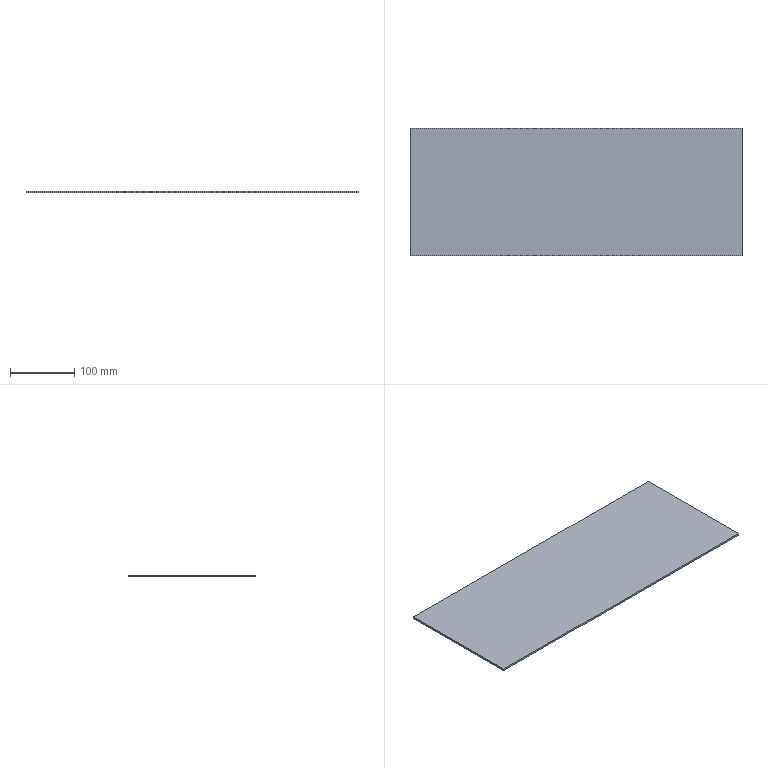Part | SolidWorks | features Extrusion 1 | 1 solid | 6 faces | box 515 x 198 x 3 mm | volume 305910 mm3 | plane 6
STEP:
#1=CARTESIAN_POINT('',(257.5,-99.,0.));
#2=VERTEX_POINT('',#1);
#3=CARTESIAN_POINT('',(257.5,99.,0.));
#4=VERTEX_POINT('',#3);
#5=CARTESIAN_POINT('',(257.5,99.,0.));
#6=DIRECTION('',(0.,1.,0.));
#7=VECTOR('',#6,1000.);
#8=LINE('',#5,#7);
#9=EDGE_CURVE('',#2,#4,#8,.T.);
#10=ORIENTED_EDGE('',*,*,#9,.T.);
#11=CARTESIAN_POINT('',(257.5,99.,3.));
#12=VERTEX_POINT('',#11);
#13=CARTESIAN_POINT('',(257.5,99.,3.));
#14=DIRECTION('',(0.,0.,-1.));
#15=VECTOR('',#14,1000.);
#16=LINE('',#13,#15);
#17=EDGE_CURVE('',#12,#4,#16,.T.);
#18=ORIENTED_EDGE('',*,*,#17,.F.);
#19=CARTESIAN_POINT('',(257.5,-99.,3.));
#20=VERTEX_POINT('',#19);
#21=CARTESIAN_POINT('',(257.5,99.,3.));
#22=DIRECTION('',(0.,1.,0.));
#23=VECTOR('',#22,1000.);
#24=LINE('',#21,#23);
#25=EDGE_CURVE('',#20,#12,#24,.T.);
#26=ORIENTED_EDGE('',*,*,#25,.F.);
#27=CARTESIAN_POINT('',(257.5,-99.,3.));
#28=DIRECTION('',(0.,0.,-1.));
#29=VECTOR('',#28,1000.);
#30=LINE('',#27,#29);
#31=EDGE_CURVE('',#20,#2,#30,.T.);
#32=ORIENTED_EDGE('',*,*,#31,.T.);
#33=EDGE_LOOP('',(#10,#18,#26,#32));
#34=FACE_OUTER_BOUND('',#33,.T.);
#35=CARTESIAN_POINT('',(257.5,99.,3.));
#36=DIRECTION('',(-1.,0.,0.));
#37=DIRECTION('',(0.,0.,1.));
#38=AXIS2_PLACEMENT_3D('',#35,#36,#37);
#39=PLANE('',#38);
#40=ADVANCED_FACE('',(#34),#39,.F.);
#41=CARTESIAN_POINT('',(-257.5,99.,0.));
#42=VERTEX_POINT('',#41);
#43=CARTESIAN_POINT('',(-257.5,99.,0.));
#44=DIRECTION('',(-1.,0.,0.));
#45=VECTOR('',#44,1000.);
#46=LINE('',#43,#45);
#47=EDGE_CURVE('',#4,#42,#46,.T.);
#48=ORIENTED_EDGE('',*,*,#47,.T.);
#49=CARTESIAN_POINT('',(-257.5,99.,3.));
#50=VERTEX_POINT('',#49);
#51=CARTESIAN_POINT('',(-257.5,99.,3.));
#52=DIRECTION('',(0.,0.,-1.));
#53=VECTOR('',#52,1000.);
#54=LINE('',#51,#53);
#55=EDGE_CURVE('',#50,#42,#54,.T.);
#56=ORIENTED_EDGE('',*,*,#55,.F.);
#57=CARTESIAN_POINT('',(-257.5,99.,3.));
#58=DIRECTION('',(-1.,0.,0.));
#59=VECTOR('',#58,1000.);
#60=LINE('',#57,#59);
#61=EDGE_CURVE('',#12,#50,#60,.T.);
#62=ORIENTED_EDGE('',*,*,#61,.F.);
#63=ORIENTED_EDGE('',*,*,#17,.T.);
#64=EDGE_LOOP('',(#48,#56,#62,#63));
#65=FACE_OUTER_BOUND('',#64,.T.);
#66=CARTESIAN_POINT('',(-257.5,99.,3.));
#67=DIRECTION('',(0.,-1.,0.));
#68=DIRECTION('',(0.,0.,-1.));
#69=AXIS2_PLACEMENT_3D('',#66,#67,#68);
#70=PLANE('',#69);
#71=ADVANCED_FACE('',(#65),#70,.F.);
#72=CARTESIAN_POINT('',(-257.5,-99.,0.));
#73=VERTEX_POINT('',#72);
#74=CARTESIAN_POINT('',(-257.5,99.,0.));
#75=DIRECTION('',(0.,-1.,0.));
#76=VECTOR('',#75,1000.);
#77=LINE('',#74,#76);
#78=EDGE_CURVE('',#42,#73,#77,.T.);
#79=ORIENTED_EDGE('',*,*,#78,.T.);
#80=CARTESIAN_POINT('',(-257.5,-99.,3.));
#81=VERTEX_POINT('',#80);
#82=CARTESIAN_POINT('',(-257.5,-99.,3.));
#83=DIRECTION('',(0.,0.,-1.));
#84=VECTOR('',#83,1000.);
#85=LINE('',#82,#84);
#86=EDGE_CURVE('',#81,#73,#85,.T.);
#87=ORIENTED_EDGE('',*,*,#86,.F.);
#88=CARTESIAN_POINT('',(-257.5,99.,3.));
#89=DIRECTION('',(0.,-1.,0.));
#90=VECTOR('',#89,1000.);
#91=LINE('',#88,#90);
#92=EDGE_CURVE('',#50,#81,#91,.T.);
#93=ORIENTED_EDGE('',*,*,#92,.F.);
#94=ORIENTED_EDGE('',*,*,#55,.T.);
#95=EDGE_LOOP('',(#79,#87,#93,#94));
#96=FACE_OUTER_BOUND('',#95,.T.);
#97=CARTESIAN_POINT('',(-257.5,99.,3.));
#98=DIRECTION('',(1.,0.,0.));
#99=DIRECTION('',(0.,0.,-1.));
#100=AXIS2_PLACEMENT_3D('',#97,#98,#99);
#101=PLANE('',#100);
#102=ADVANCED_FACE('',(#96),#101,.F.);
#103=CARTESIAN_POINT('',(-257.5,-99.,0.));
#104=DIRECTION('',(1.,0.,0.));
#105=VECTOR('',#104,1000.);
#106=LINE('',#103,#105);
#107=EDGE_CURVE('',#73,#2,#106,.T.);
#108=ORIENTED_EDGE('',*,*,#107,.T.);
#109=ORIENTED_EDGE('',*,*,#31,.F.);
#110=CARTESIAN_POINT('',(-257.5,-99.,3.));
#111=DIRECTION('',(1.,0.,0.));
#112=VECTOR('',#111,1000.);
#113=LINE('',#110,#112);
#114=EDGE_CURVE('',#81,#20,#113,.T.);
#115=ORIENTED_EDGE('',*,*,#114,.F.);
#116=ORIENTED_EDGE('',*,*,#86,.T.);
#117=EDGE_LOOP('',(#108,#109,#115,#116));
#118=FACE_OUTER_BOUND('',#117,.T.);
#119=CARTESIAN_POINT('',(-257.5,-99.,3.));
#120=DIRECTION('',(0.,1.,0.));
#121=DIRECTION('',(0.,0.,1.));
#122=AXIS2_PLACEMENT_3D('',#119,#120,#121);
#123=PLANE('',#122);
#124=ADVANCED_FACE('',(#118),#123,.F.);
#125=ORIENTED_EDGE('',*,*,#25,.T.);
#126=ORIENTED_EDGE('',*,*,#61,.T.);
#127=ORIENTED_EDGE('',*,*,#92,.T.);
#128=ORIENTED_EDGE('',*,*,#114,.T.);
#129=EDGE_LOOP('',(#125,#126,#127,#128));
#130=FACE_OUTER_BOUND('',#129,.T.);
#131=CARTESIAN_POINT('',(0.,0.,3.));
#132=DIRECTION('',(0.,0.,1.));
#133=DIRECTION('',(1.,0.,0.));
#134=AXIS2_PLACEMENT_3D('',#131,#132,#133);
#135=PLANE('',#134);
#136=ADVANCED_FACE('',(#130),#135,.T.);
#137=ORIENTED_EDGE('',*,*,#9,.F.);
#138=ORIENTED_EDGE('',*,*,#107,.F.);
#139=ORIENTED_EDGE('',*,*,#78,.F.);
#140=ORIENTED_EDGE('',*,*,#47,.F.);
#141=EDGE_LOOP('',(#137,#138,#139,#140));
#142=FACE_OUTER_BOUND('',#141,.T.);
#143=CARTESIAN_POINT('',(0.,0.,0.));
#144=DIRECTION('',(0.,0.,1.));
#145=DIRECTION('',(1.,0.,0.));
#146=AXIS2_PLACEMENT_3D('',#143,#144,#145);
#147=PLANE('',#146);
#148=ADVANCED_FACE('',(#142),#147,.F.);
#149=CLOSED_SHELL('',(#40,#71,#102,#124,#136,#148));
#150=MANIFOLD_SOLID_BREP('',#149);
#151=CARTESIAN_POINT('',(0.,0.,0.));
#152=DIRECTION('',(0.,0.,1.));
#153=DIRECTION('',(1.,0.,0.));
#154=AXIS2_PLACEMENT_3D('',#151,#152,#153);
#155=(LENGTH_UNIT()NAMED_UNIT(*)SI_UNIT(.MILLI.,.METRE.));
#156=UNCERTAINTY_MEASURE_WITH_UNIT(LENGTH_MEASURE(0.00001),#155,'','');
#157=(NAMED_UNIT(*)PLANE_ANGLE_UNIT()SI_UNIT($,.RADIAN.));
#158=(NAMED_UNIT(*)SI_UNIT($,.STERADIAN.)SOLID_ANGLE_UNIT());
#159=(GEOMETRIC_REPRESENTATION_CONTEXT(3)GLOBAL_UNCERTAINTY_ASSIGNED_CONTEXT((#156))GLOBAL_UNIT_ASSIGNED_CONTEXT((#155,#157,#158))REPRESENTATION_CONTEXT('',''));
#160=ADVANCED_BREP_SHAPE_REPRESENTATION('',(#150,#154),#159);